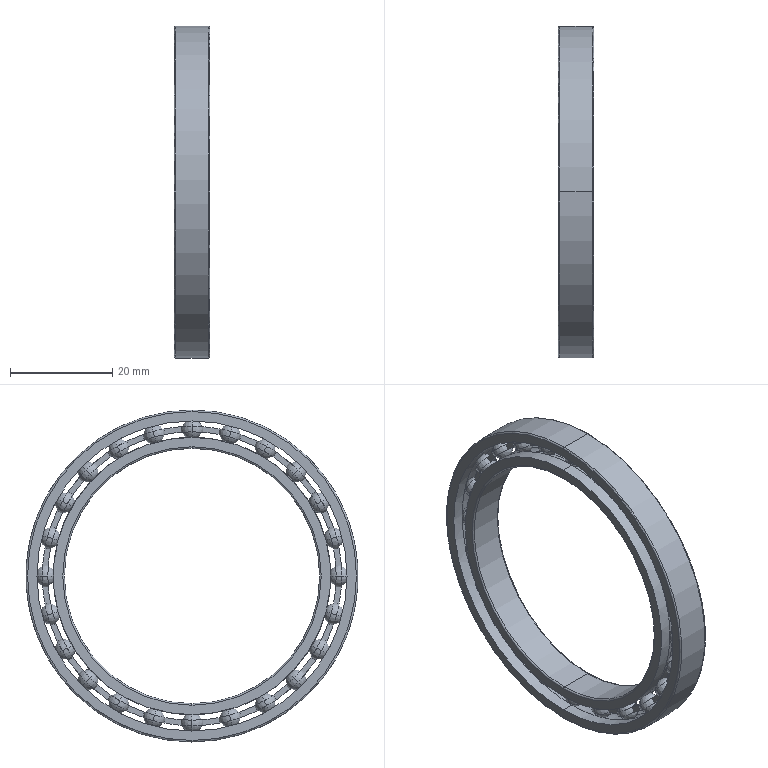Part | SolidWorks | 1 solid | 340 faces | box 7 x 65 x 65 mm | volume 6140 mm3 | sphere 192 | torus 80 | plane 52 | cylinder 16 | commonest cylinder face diameters 54.3 x4 60.7 x4 50 x2 56.409 x2 58.591 x2 65 x2